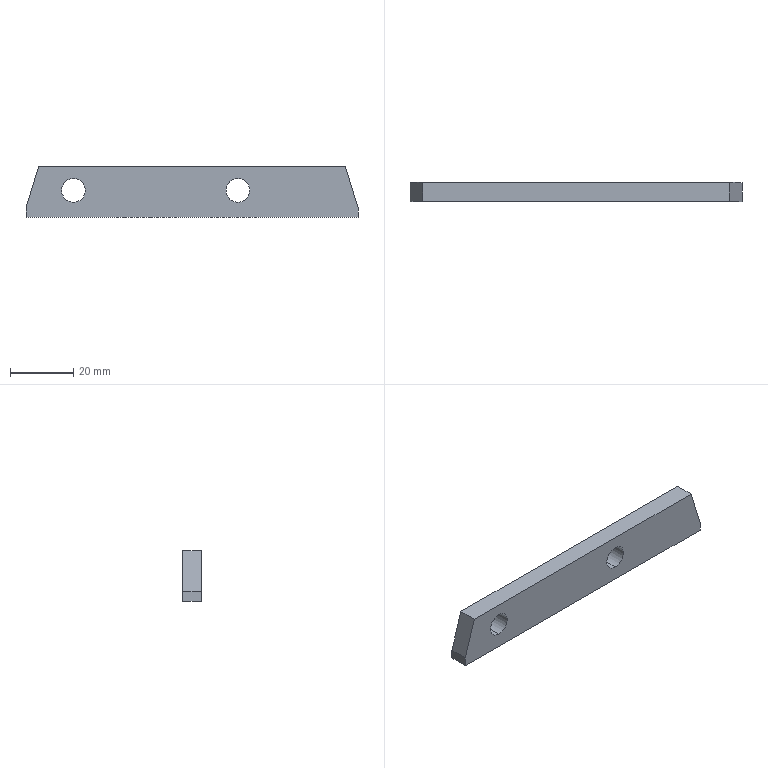Part | 1 solid | 12 faces | box 105 x 6 x 16 mm | volume 9238 mm3 | plane 8 | cylinder 4 | commonest cylinder face diameters 7.5 x4
STEP:
#1=CARTESIAN_POINT('',(11.,0.,-11.25));
#2=VERTEX_POINT('',#1);
#3=CARTESIAN_POINT('',(11.,0.,-3.75));
#4=VERTEX_POINT('',#3);
#5=CARTESIAN_POINT('',(11.,0.,-7.5));
#6=DIRECTION('',(0.,1.,0.));
#7=DIRECTION('',(0.,0.,-1.));
#8=AXIS2_PLACEMENT_3D('',#5,#6,#7);
#9=CIRCLE('',#8,3.75);
#10=EDGE_CURVE('',#2,#4,#9,.T.);
#11=ORIENTED_EDGE('',*,*,#10,.F.);
#12=CARTESIAN_POINT('',(11.,6.,-11.25));
#13=VERTEX_POINT('',#12);
#14=CARTESIAN_POINT('',(11.,0.,-11.25));
#15=DIRECTION('',(0.,1.,0.));
#16=VECTOR('',#15,1000.);
#17=LINE('',#14,#16);
#18=EDGE_CURVE('',#2,#13,#17,.T.);
#19=ORIENTED_EDGE('',*,*,#18,.T.);
#20=CARTESIAN_POINT('',(11.,6.,-3.75));
#21=VERTEX_POINT('',#20);
#22=CARTESIAN_POINT('',(11.,6.,-7.5));
#23=DIRECTION('',(0.,1.,0.));
#24=DIRECTION('',(0.,0.,-1.));
#25=AXIS2_PLACEMENT_3D('',#22,#23,#24);
#26=CIRCLE('',#25,3.75);
#27=EDGE_CURVE('',#13,#21,#26,.T.);
#28=ORIENTED_EDGE('',*,*,#27,.T.);
#29=CARTESIAN_POINT('',(11.,0.,-3.75));
#30=DIRECTION('',(0.,1.,0.));
#31=VECTOR('',#30,1000.);
#32=LINE('',#29,#31);
#33=EDGE_CURVE('',#4,#21,#32,.T.);
#34=ORIENTED_EDGE('',*,*,#33,.F.);
#35=EDGE_LOOP('',(#11,#19,#28,#34));
#36=FACE_OUTER_BOUND('',#35,.T.);
#37=CARTESIAN_POINT('',(11.,0.,-7.5));
#38=DIRECTION('',(0.,1.,0.));
#39=DIRECTION('',(0.,0.,1.));
#40=AXIS2_PLACEMENT_3D('',#37,#38,#39);
#41=CYLINDRICAL_SURFACE('',#40,3.75);
#42=ADVANCED_FACE('',(#36),#41,.F.);
#43=CARTESIAN_POINT('',(63.,0.,-11.25));
#44=VERTEX_POINT('',#43);
#45=CARTESIAN_POINT('',(63.,0.,-3.75));
#46=VERTEX_POINT('',#45);
#47=CARTESIAN_POINT('',(63.,0.,-7.5));
#48=DIRECTION('',(0.,1.,0.));
#49=DIRECTION('',(0.,0.,-1.));
#50=AXIS2_PLACEMENT_3D('',#47,#48,#49);
#51=CIRCLE('',#50,3.75);
#52=EDGE_CURVE('',#44,#46,#51,.T.);
#53=ORIENTED_EDGE('',*,*,#52,.F.);
#54=CARTESIAN_POINT('',(63.,6.,-11.25));
#55=VERTEX_POINT('',#54);
#56=CARTESIAN_POINT('',(63.,0.,-11.25));
#57=DIRECTION('',(0.,1.,0.));
#58=VECTOR('',#57,1000.);
#59=LINE('',#56,#58);
#60=EDGE_CURVE('',#44,#55,#59,.T.);
#61=ORIENTED_EDGE('',*,*,#60,.T.);
#62=CARTESIAN_POINT('',(63.,6.,-3.75));
#63=VERTEX_POINT('',#62);
#64=CARTESIAN_POINT('',(63.,6.,-7.5));
#65=DIRECTION('',(0.,1.,0.));
#66=DIRECTION('',(0.,0.,-1.));
#67=AXIS2_PLACEMENT_3D('',#64,#65,#66);
#68=CIRCLE('',#67,3.75);
#69=EDGE_CURVE('',#55,#63,#68,.T.);
#70=ORIENTED_EDGE('',*,*,#69,.T.);
#71=CARTESIAN_POINT('',(63.,0.,-3.75));
#72=DIRECTION('',(0.,1.,0.));
#73=VECTOR('',#72,1000.);
#74=LINE('',#71,#73);
#75=EDGE_CURVE('',#46,#63,#74,.T.);
#76=ORIENTED_EDGE('',*,*,#75,.F.);
#77=EDGE_LOOP('',(#53,#61,#70,#76));
#78=FACE_OUTER_BOUND('',#77,.T.);
#79=CARTESIAN_POINT('',(63.,0.,-7.5));
#80=DIRECTION('',(0.,1.,0.));
#81=DIRECTION('',(0.,0.,1.));
#82=AXIS2_PLACEMENT_3D('',#79,#80,#81);
#83=CYLINDRICAL_SURFACE('',#82,3.75);
#84=ADVANCED_FACE('',(#78),#83,.F.);
#85=CARTESIAN_POINT('',(-4.,6.,-13.));
#86=VERTEX_POINT('',#85);
#87=CARTESIAN_POINT('',(0.,6.,0.));
#88=VERTEX_POINT('',#87);
#89=CARTESIAN_POINT('',(-4.,6.,-13.));
#90=DIRECTION('',(0.2941,0.,0.9558));
#91=VECTOR('',#90,1000.);
#92=LINE('',#89,#91);
#93=EDGE_CURVE('',#86,#88,#92,.T.);
#94=ORIENTED_EDGE('',*,*,#93,.F.);
#95=CARTESIAN_POINT('',(-4.,0.,-13.));
#96=VERTEX_POINT('',#95);
#97=CARTESIAN_POINT('',(-4.,0.,-13.));
#98=DIRECTION('',(0.,1.,0.));
#99=VECTOR('',#98,1000.);
#100=LINE('',#97,#99);
#101=EDGE_CURVE('',#96,#86,#100,.T.);
#102=ORIENTED_EDGE('',*,*,#101,.F.);
#103=CARTESIAN_POINT('',(0.,0.,0.));
#104=VERTEX_POINT('',#103);
#105=CARTESIAN_POINT('',(-4.,0.,-13.));
#106=DIRECTION('',(0.2941,0.,0.9558));
#107=VECTOR('',#106,1000.);
#108=LINE('',#105,#107);
#109=EDGE_CURVE('',#96,#104,#108,.T.);
#110=ORIENTED_EDGE('',*,*,#109,.T.);
#111=CARTESIAN_POINT('',(0.,0.,0.));
#112=DIRECTION('',(0.,1.,0.));
#113=VECTOR('',#112,1000.);
#114=LINE('',#111,#113);
#115=EDGE_CURVE('',#104,#88,#114,.T.);
#116=ORIENTED_EDGE('',*,*,#115,.T.);
#117=EDGE_LOOP('',(#94,#102,#110,#116));
#118=FACE_OUTER_BOUND('',#117,.T.);
#119=CARTESIAN_POINT('',(-4.,0.,-13.));
#120=DIRECTION('',(-0.9558,0.,0.2941));
#121=DIRECTION('',(0.2941,0.,0.9558));
#122=AXIS2_PLACEMENT_3D('',#119,#120,#121);
#123=PLANE('',#122);
#124=ADVANCED_FACE('',(#118),#123,.T.);
#125=CARTESIAN_POINT('',(-4.,6.,-16.));
#126=VERTEX_POINT('',#125);
#127=CARTESIAN_POINT('',(-4.,6.,-16.));
#128=DIRECTION('',(0.,0.,1.));
#129=VECTOR('',#128,1000.);
#130=LINE('',#127,#129);
#131=EDGE_CURVE('',#126,#86,#130,.T.);
#132=ORIENTED_EDGE('',*,*,#131,.F.);
#133=CARTESIAN_POINT('',(-4.,0.,-16.));
#134=VERTEX_POINT('',#133);
#135=CARTESIAN_POINT('',(-4.,0.,-16.));
#136=DIRECTION('',(0.,1.,0.));
#137=VECTOR('',#136,1000.);
#138=LINE('',#135,#137);
#139=EDGE_CURVE('',#134,#126,#138,.T.);
#140=ORIENTED_EDGE('',*,*,#139,.F.);
#141=CARTESIAN_POINT('',(-4.,0.,-16.));
#142=DIRECTION('',(0.,0.,1.));
#143=VECTOR('',#142,1000.);
#144=LINE('',#141,#143);
#145=EDGE_CURVE('',#134,#96,#144,.T.);
#146=ORIENTED_EDGE('',*,*,#145,.T.);
#147=ORIENTED_EDGE('',*,*,#101,.T.);
#148=EDGE_LOOP('',(#132,#140,#146,#147));
#149=FACE_OUTER_BOUND('',#148,.T.);
#150=CARTESIAN_POINT('',(-4.,0.,-16.));
#151=DIRECTION('',(-1.,0.,0.));
#152=DIRECTION('',(0.,0.,1.));
#153=AXIS2_PLACEMENT_3D('',#150,#151,#152);
#154=PLANE('',#153);
#155=ADVANCED_FACE('',(#149),#154,.T.);
#156=CARTESIAN_POINT('',(101.,6.,-16.));
#157=VERTEX_POINT('',#156);
#158=CARTESIAN_POINT('',(101.,6.,-16.));
#159=DIRECTION('',(-1.,0.,0.));
#160=VECTOR('',#159,1000.);
#161=LINE('',#158,#160);
#162=EDGE_CURVE('',#157,#126,#161,.T.);
#163=ORIENTED_EDGE('',*,*,#162,.F.);
#164=CARTESIAN_POINT('',(101.,0.,-16.));
#165=VERTEX_POINT('',#164);
#166=CARTESIAN_POINT('',(101.,0.,-16.));
#167=DIRECTION('',(0.,1.,0.));
#168=VECTOR('',#167,1000.);
#169=LINE('',#166,#168);
#170=EDGE_CURVE('',#165,#157,#169,.T.);
#171=ORIENTED_EDGE('',*,*,#170,.F.);
#172=CARTESIAN_POINT('',(101.,0.,-16.));
#173=DIRECTION('',(-1.,0.,0.));
#174=VECTOR('',#173,1000.);
#175=LINE('',#172,#174);
#176=EDGE_CURVE('',#165,#134,#175,.T.);
#177=ORIENTED_EDGE('',*,*,#176,.T.);
#178=ORIENTED_EDGE('',*,*,#139,.T.);
#179=EDGE_LOOP('',(#163,#171,#177,#178));
#180=FACE_OUTER_BOUND('',#179,.T.);
#181=CARTESIAN_POINT('',(101.,0.,-16.));
#182=DIRECTION('',(0.,0.,-1.));
#183=DIRECTION('',(-1.,0.,0.));
#184=AXIS2_PLACEMENT_3D('',#181,#182,#183);
#185=PLANE('',#184);
#186=ADVANCED_FACE('',(#180),#185,.T.);
#187=CARTESIAN_POINT('',(101.,6.,-13.));
#188=VERTEX_POINT('',#187);
#189=CARTESIAN_POINT('',(101.,6.,-13.));
#190=DIRECTION('',(0.,0.,-1.));
#191=VECTOR('',#190,1000.);
#192=LINE('',#189,#191);
#193=EDGE_CURVE('',#188,#157,#192,.T.);
#194=ORIENTED_EDGE('',*,*,#193,.F.);
#195=CARTESIAN_POINT('',(101.,0.,-13.));
#196=VERTEX_POINT('',#195);
#197=CARTESIAN_POINT('',(101.,0.,-13.));
#198=DIRECTION('',(0.,1.,0.));
#199=VECTOR('',#198,1000.);
#200=LINE('',#197,#199);
#201=EDGE_CURVE('',#196,#188,#200,.T.);
#202=ORIENTED_EDGE('',*,*,#201,.F.);
#203=CARTESIAN_POINT('',(101.,0.,-13.));
#204=DIRECTION('',(0.,0.,-1.));
#205=VECTOR('',#204,1000.);
#206=LINE('',#203,#205);
#207=EDGE_CURVE('',#196,#165,#206,.T.);
#208=ORIENTED_EDGE('',*,*,#207,.T.);
#209=ORIENTED_EDGE('',*,*,#170,.T.);
#210=EDGE_LOOP('',(#194,#202,#208,#209));
#211=FACE_OUTER_BOUND('',#210,.T.);
#212=CARTESIAN_POINT('',(101.,0.,-13.));
#213=DIRECTION('',(1.,0.,0.));
#214=DIRECTION('',(0.,0.,-1.));
#215=AXIS2_PLACEMENT_3D('',#212,#213,#214);
#216=PLANE('',#215);
#217=ADVANCED_FACE('',(#211),#216,.T.);
#218=CARTESIAN_POINT('',(97.,6.,0.));
#219=VERTEX_POINT('',#218);
#220=CARTESIAN_POINT('',(97.,6.,0.));
#221=DIRECTION('',(0.2941,0.,-0.9558));
#222=VECTOR('',#221,1000.);
#223=LINE('',#220,#222);
#224=EDGE_CURVE('',#219,#188,#223,.T.);
#225=ORIENTED_EDGE('',*,*,#224,.F.);
#226=CARTESIAN_POINT('',(97.,0.,0.));
#227=VERTEX_POINT('',#226);
#228=CARTESIAN_POINT('',(97.,0.,0.));
#229=DIRECTION('',(0.,1.,0.));
#230=VECTOR('',#229,1000.);
#231=LINE('',#228,#230);
#232=EDGE_CURVE('',#227,#219,#231,.T.);
#233=ORIENTED_EDGE('',*,*,#232,.F.);
#234=CARTESIAN_POINT('',(97.,0.,0.));
#235=DIRECTION('',(0.2941,0.,-0.9558));
#236=VECTOR('',#235,1000.);
#237=LINE('',#234,#236);
#238=EDGE_CURVE('',#227,#196,#237,.T.);
#239=ORIENTED_EDGE('',*,*,#238,.T.);
#240=ORIENTED_EDGE('',*,*,#201,.T.);
#241=EDGE_LOOP('',(#225,#233,#239,#240));
#242=FACE_OUTER_BOUND('',#241,.T.);
#243=CARTESIAN_POINT('',(97.,0.,0.));
#244=DIRECTION('',(0.9558,0.,0.2941));
#245=DIRECTION('',(0.2941,0.,-0.9558));
#246=AXIS2_PLACEMENT_3D('',#243,#244,#245);
#247=PLANE('',#246);
#248=ADVANCED_FACE('',(#242),#247,.T.);
#249=CARTESIAN_POINT('',(0.,6.,0.));
#250=DIRECTION('',(1.,0.,0.));
#251=VECTOR('',#250,1000.);
#252=LINE('',#249,#251);
#253=EDGE_CURVE('',#88,#219,#252,.T.);
#254=ORIENTED_EDGE('',*,*,#253,.F.);
#255=ORIENTED_EDGE('',*,*,#115,.F.);
#256=CARTESIAN_POINT('',(0.,0.,0.));
#257=DIRECTION('',(1.,0.,0.));
#258=VECTOR('',#257,1000.);
#259=LINE('',#256,#258);
#260=EDGE_CURVE('',#104,#227,#259,.T.);
#261=ORIENTED_EDGE('',*,*,#260,.T.);
#262=ORIENTED_EDGE('',*,*,#232,.T.);
#263=EDGE_LOOP('',(#254,#255,#261,#262));
#264=FACE_OUTER_BOUND('',#263,.T.);
#265=CARTESIAN_POINT('',(0.,0.,0.));
#266=DIRECTION('',(0.,0.,1.));
#267=DIRECTION('',(1.,0.,0.));
#268=AXIS2_PLACEMENT_3D('',#265,#266,#267);
#269=PLANE('',#268);
#270=ADVANCED_FACE('',(#264),#269,.T.);
#271=CARTESIAN_POINT('',(11.,0.,-7.5));
#272=DIRECTION('',(0.,1.,0.));
#273=DIRECTION('',(0.,0.,-1.));
#274=AXIS2_PLACEMENT_3D('',#271,#272,#273);
#275=CIRCLE('',#274,3.75);
#276=EDGE_CURVE('',#4,#2,#275,.T.);
#277=ORIENTED_EDGE('',*,*,#276,.T.);
#278=ORIENTED_EDGE('',*,*,#10,.T.);
#279=EDGE_LOOP('',(#277,#278));
#280=FACE_BOUND('',#279,.T.);
#281=CARTESIAN_POINT('',(63.,0.,-7.5));
#282=DIRECTION('',(0.,1.,0.));
#283=DIRECTION('',(0.,0.,-1.));
#284=AXIS2_PLACEMENT_3D('',#281,#282,#283);
#285=CIRCLE('',#284,3.75);
#286=EDGE_CURVE('',#46,#44,#285,.T.);
#287=ORIENTED_EDGE('',*,*,#286,.T.);
#288=ORIENTED_EDGE('',*,*,#52,.T.);
#289=EDGE_LOOP('',(#287,#288));
#290=FACE_BOUND('',#289,.T.);
#291=ORIENTED_EDGE('',*,*,#109,.F.);
#292=ORIENTED_EDGE('',*,*,#145,.F.);
#293=ORIENTED_EDGE('',*,*,#176,.F.);
#294=ORIENTED_EDGE('',*,*,#207,.F.);
#295=ORIENTED_EDGE('',*,*,#238,.F.);
#296=ORIENTED_EDGE('',*,*,#260,.F.);
#297=EDGE_LOOP('',(#291,#292,#293,#294,#295,#296));
#298=FACE_OUTER_BOUND('',#297,.T.);
#299=CARTESIAN_POINT('',(0.,0.,0.));
#300=DIRECTION('',(0.,1.,0.));
#301=DIRECTION('',(0.,0.,1.));
#302=AXIS2_PLACEMENT_3D('',#299,#300,#301);
#303=PLANE('',#302);
#304=ADVANCED_FACE('',(#280,#290,#298),#303,.F.);
#305=CARTESIAN_POINT('',(11.,6.,-7.5));
#306=DIRECTION('',(0.,1.,0.));
#307=DIRECTION('',(0.,0.,-1.));
#308=AXIS2_PLACEMENT_3D('',#305,#306,#307);
#309=CIRCLE('',#308,3.75);
#310=EDGE_CURVE('',#21,#13,#309,.T.);
#311=ORIENTED_EDGE('',*,*,#310,.F.);
#312=ORIENTED_EDGE('',*,*,#27,.F.);
#313=EDGE_LOOP('',(#311,#312));
#314=FACE_BOUND('',#313,.T.);
#315=CARTESIAN_POINT('',(63.,6.,-7.5));
#316=DIRECTION('',(0.,1.,0.));
#317=DIRECTION('',(0.,0.,-1.));
#318=AXIS2_PLACEMENT_3D('',#315,#316,#317);
#319=CIRCLE('',#318,3.75);
#320=EDGE_CURVE('',#63,#55,#319,.T.);
#321=ORIENTED_EDGE('',*,*,#320,.F.);
#322=ORIENTED_EDGE('',*,*,#69,.F.);
#323=EDGE_LOOP('',(#321,#322));
#324=FACE_BOUND('',#323,.T.);
#325=ORIENTED_EDGE('',*,*,#93,.T.);
#326=ORIENTED_EDGE('',*,*,#253,.T.);
#327=ORIENTED_EDGE('',*,*,#224,.T.);
#328=ORIENTED_EDGE('',*,*,#193,.T.);
#329=ORIENTED_EDGE('',*,*,#162,.T.);
#330=ORIENTED_EDGE('',*,*,#131,.T.);
#331=EDGE_LOOP('',(#325,#326,#327,#328,#329,#330));
#332=FACE_OUTER_BOUND('',#331,.T.);
#333=CARTESIAN_POINT('',(0.,6.,0.));
#334=DIRECTION('',(0.,1.,0.));
#335=DIRECTION('',(0.,0.,1.));
#336=AXIS2_PLACEMENT_3D('',#333,#334,#335);
#337=PLANE('',#336);
#338=ADVANCED_FACE('',(#314,#324,#332),#337,.T.);
#339=ORIENTED_EDGE('',*,*,#60,.F.);
#340=ORIENTED_EDGE('',*,*,#286,.F.);
#341=ORIENTED_EDGE('',*,*,#75,.T.);
#342=ORIENTED_EDGE('',*,*,#320,.T.);
#343=EDGE_LOOP('',(#339,#340,#341,#342));
#344=FACE_OUTER_BOUND('',#343,.T.);
#345=CARTESIAN_POINT('',(63.,0.,-7.5));
#346=DIRECTION('',(0.,1.,0.));
#347=DIRECTION('',(0.,0.,1.));
#348=AXIS2_PLACEMENT_3D('',#345,#346,#347);
#349=CYLINDRICAL_SURFACE('',#348,3.75);
#350=ADVANCED_FACE('',(#344),#349,.F.);
#351=ORIENTED_EDGE('',*,*,#18,.F.);
#352=ORIENTED_EDGE('',*,*,#276,.F.);
#353=ORIENTED_EDGE('',*,*,#33,.T.);
#354=ORIENTED_EDGE('',*,*,#310,.T.);
#355=EDGE_LOOP('',(#351,#352,#353,#354));
#356=FACE_OUTER_BOUND('',#355,.T.);
#357=CARTESIAN_POINT('',(11.,0.,-7.5));
#358=DIRECTION('',(0.,1.,0.));
#359=DIRECTION('',(0.,0.,1.));
#360=AXIS2_PLACEMENT_3D('',#357,#358,#359);
#361=CYLINDRICAL_SURFACE('',#360,3.75);
#362=ADVANCED_FACE('',(#356),#361,.F.);
#363=CLOSED_SHELL('',(#42,#84,#124,#155,#186,#217,#248,#270,#304,#338,#350,#362));
#364=MANIFOLD_SOLID_BREP('',#363);
#365=CARTESIAN_POINT('',(0.,0.,0.));
#366=DIRECTION('',(0.,0.,1.));
#367=DIRECTION('',(1.,0.,0.));
#368=AXIS2_PLACEMENT_3D('',#365,#366,#367);
#369=(LENGTH_UNIT()NAMED_UNIT(*)SI_UNIT(.MILLI.,.METRE.));
#370=UNCERTAINTY_MEASURE_WITH_UNIT(LENGTH_MEASURE(0.00001),#369,'','');
#371=(NAMED_UNIT(*)PLANE_ANGLE_UNIT()SI_UNIT($,.RADIAN.));
#372=(NAMED_UNIT(*)SI_UNIT($,.STERADIAN.)SOLID_ANGLE_UNIT());
#373=(GEOMETRIC_REPRESENTATION_CONTEXT(3)GLOBAL_UNCERTAINTY_ASSIGNED_CONTEXT((#370))GLOBAL_UNIT_ASSIGNED_CONTEXT((#369,#371,#372))REPRESENTATION_CONTEXT('',''));
#374=ADVANCED_BREP_SHAPE_REPRESENTATION('',(#364,#368),#373);